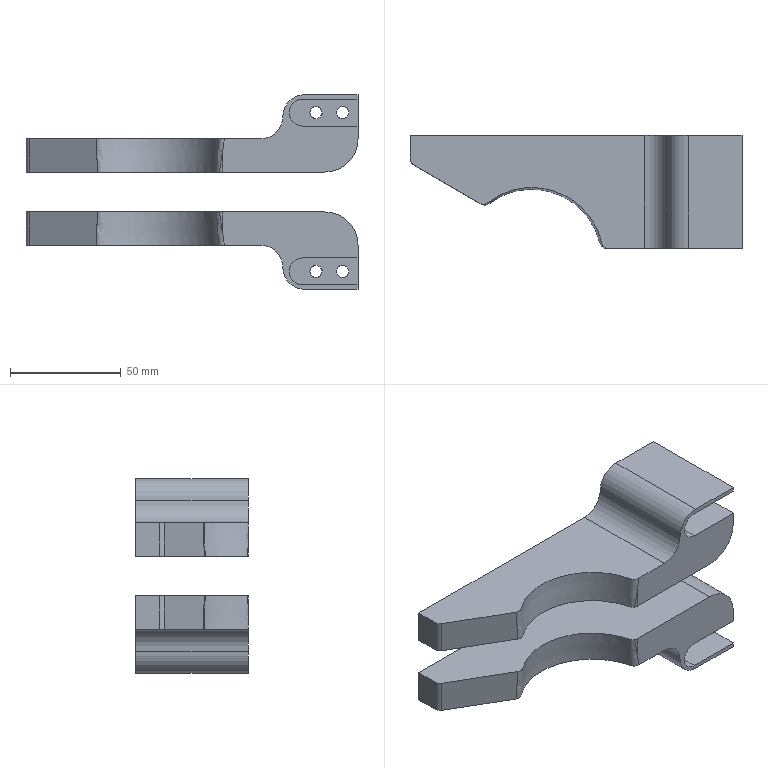NC program | NX | posted with a generic post | part box 150 x 51 x 88 mm
Lines 43 to 1068 of 21230:
(ADAPTIVE_MILLING_COPY , TOOL : D12C)
N72 T12 M6
N74 G54
N76 G17 G0 G90 X-87.243 Y2.564 S9500 M3
N78 G43 Z30. H12
N80 Z-14.
N82 G94 G1 Z-17. F1000.
N84 X-85.489 Y2.014 F3000.
N86 G3 X-84.076 Y2.564 R1.22
N88 X-83.366 Y5.337 R7.621
N90 X-83.032 Y14.477 R92.487
N92 G2 X-82.959 Y17.999 R38.072
N94 X-79.583 Y22.839 R7.317
N96 X-73.241 Y24.982 R15.248
N98 X-63.509 Y25.457 R81.144
N100 G1 X-62.234 Y25.466
N102 X-60.584 Y25.474
N104 X-58.409 Y25.479
N106 X-55.034 Y25.483
N108 X-47.909 Y25.485
N110 X74.716 Y25.478
N112 X74.791 Y25.477
N114 X74.941 Y25.472
N116 X75.091 Y25.462
N118 G2 X80.055 Y22.427 R7.028
N120 X82.397 Y16.243 R14.195
N122 X82.947 Y7.042 R66.047
N124 G1 X82.959 Y5.918
N126 X82.968 Y4.568
N128 X82.976 Y2.843
N130 X82.982 Y0.593
N132 X82.986 Y-2.932
N134 X82.988 Y-10.957
N136 G2 X82.946 Y-17.856 R138.275
N138 X79.66 Y-22.754 R7.252
N140 X73.342 Y-24.96 R14.994
N142 X64.586 Y-25.446 R70.223
N144 G1 X63.461 Y-25.458
N146 X62.111 Y-25.467
N148 X60.536 Y-25.475
N150 X58.286 Y-25.48
N152 X54.911 Y-25.484
N154 X47.561 Y-25.486
N156 X-74.689 Y-25.485
N158 X-74.764
N160 X-74.839 Y-25.483
N162 X-74.988 Y-25.476
N164 X-75.138 Y-25.465
N166 G2 X-80.128 Y-22.335 R7.093
N168 X-82.394 Y-16.278 R14.265
N170 X-82.95 Y-7.078 R64.861
N172 X-82.909 Y0.045 R99.947
N174 G3 X-82.049 Y14.411 R129.844
N176 G2 X-81.128 Y17.792 R9.852
N178 X-76.298 Y23.504 R6.212
N180 X-62.095 Y24.43 R100.62
N182 G1 X-60.82 Y24.443
N184 X-59.32 Y24.453
N186 X-57.52 Y24.461
N188 X-55.12 Y24.467
N190 X-51.595 Y24.471
N192 X-44.92 Y24.473
N194 X71.33 Y24.467
N196 X71.48 Y24.466
N198 X71.705 Y24.458
N200 X71.855 Y24.451
N202 G2 X78.937 Y20.113 R9.119
N204 X81.352 Y13.152 R17.438
N206 X81.922 Y3.726 R73.479
N208 X81.951 Y-14.498 R846.878
N210 X81.136 Y-17.623 R10.548
N212 X76.298 Y-23.504 R6.215
N214 X61.795 Y-24.434 R102.394
N216 G1 X60.595 Y-24.445
N218 X59.02 Y-24.455
N220 X57.145 Y-24.463
N222 X54.595 Y-24.469
N224 X50.77 Y-24.473
N226 X42.745 Y-24.475
N228 X-71.33 Y-24.474
N230 X-71.48 Y-24.472
N232 X-71.705 Y-24.465
N234 X-71.855 Y-24.458
N236 G2 X-78.938 Y-20.121 R9.12
N238 X-81.361 Y-13.085 R17.42
N240 X-81.615 Y2.256 R70.947
N242 G3 X-81.146 Y17.535 R168.471
N244 G1 X-81.129 Y17.684
N246 X-81.146 Y17.535
N248 X-81.15 Y17.465
N250 Y11.278
N252 G2 X-81.277 Y-2.863 R390.887
N254 G3 X-80.682 Y-12.884 R63.102
N256 X-78.284 Y-19.291 R15.229
N258 X-72.558 Y-23.014 R9.886
N260 X-65.493 Y-23.797 R31.227
N262 X-51.093 Y-23.867 R747.498
N264 G1 X-11.568 Y-23.868
N266 X-11.193 Y-23.869
N268 X54.282 Y-23.87
N270 X59.682 Y-23.846
N272 G3 X68.172 Y-23.65 R287.309
N274 G1 X74.965
N276 X75.035 Y-23.646
N278 X74.965 Y-23.65
N280 X51.025
N282 X50.975 Y-23.648
N284 G2 X46.571 Y-23.171 R50.175
N286 G3 X36.303 Y-22.893 R128.49
N288 G1 X34.053 Y-22.887
N290 X30.528 Y-22.883
N292 X22.578 Y-22.881
N294 X-7.947
N296 X-8.697 Y-22.877
N298 X-9.747 Y-22.875
N300 X-10.197
N302 X-11.022 Y-22.872
N304 X-11.847
N306 X-12.897 Y-22.87
N308 X-13.722 Y-22.871
N310 X-14.622 Y-22.869
N312 X-15.822 Y-22.87
N314 X-16.497 Y-22.869
N316 X-17.772 Y-22.87
N318 X-18.222
N320 X-18.972 Y-22.869
N322 X-20.022 Y-22.87
N324 X-20.772 Y-22.868
N326 X-22.047 Y-22.87
N328 X-23.022 Y-22.867
N330 X-24.147 Y-22.87
N332 X-24.897 Y-22.868
N334 X-25.872 Y-22.869
N336 X-26.397
N338 X-27.147 Y-22.867
N340 X-27.897 Y-22.868
N342 X-29.247 Y-22.866
N344 X-29.697
N346 X-30.597 Y-22.868
N348 X-31.572 Y-22.866
N350 X-32.472 Y-22.868
N352 X-33.222 Y-22.867
N354 X-34.497 Y-22.869
N356 X-35.547 Y-22.866
N358 X-36.522 Y-22.868
N360 X-37.497 Y-22.867
N362 X-38.472 Y-22.869
N364 X-39.522 Y-22.866
N366 X-40.497 Y-22.868
N368 X-41.547 Y-22.866
N370 X-42.447 Y-22.868
N372 X-43.272 Y-22.867
N374 X-44.397 Y-22.869
N376 X-45.222 Y-22.867
N378 X-46.197 Y-22.868
N380 X-47.172 Y-22.866
N382 X-47.922 Y-22.867
N384 X-49.197 Y-22.866
N386 X-49.647 Y-22.865
N388 X-50.322 Y-22.867
N390 X-51.297 Y-22.865
N392 X-51.822 Y-22.866
N394 X-52.497 Y-22.867
N396 X-53.547 Y-22.865
N398 X-54.222 Y-22.866
N400 X-55.347 Y-22.864
N402 X-55.797 Y-22.863
N404 G2 X-67.343 Y-22.645 R181.656
N406 X-72.93 Y-21.333 R15.227
N408 X-78.322 Y-15.229 R11.546
N410 X-79.985 Y-7.412 R25.774
N412 X-80.19 Y-0.893 R100.233
N414 G1 X-80.206 Y-0.82
N416 X-80.226 Y-0.748
N418 X-80.251 Y-0.677
N420 X-80.279 Y-0.607
N422 X-80.31 Y-0.539
N424 X-80.324 Y-0.514
N426 X-80.364 Y-0.45
N428 G2 X-79.856 Y-2.236 R3.949
N430 G3 X-79.127 Y-9.247 R243.86
N432 X-76.81 Y-16.247 R18.289
N434 X-69.838 Y-21.221 R11.574
N436 X-62.639 Y-22.142 R31.464
N438 X-40.815 Y-22.267 R842.14
N440 G1 X-39.99 Y-22.265
N442 X-38.715 Y-22.268
N444 X-38.265 Y-22.267
N446 X-36.615 Y-22.27
N448 X-35.715 Y-22.267
N450 X-35.19 Y-22.268
N452 X-33.69 Y-22.265
N454 X-32.865 Y-22.267
N456 X-32.19 Y-22.266
N458 X-31.665 Y-22.267
N460 X-31.14 Y-22.266
N462 X-30.765 Y-22.267
N464 X-29.565 Y-22.265
N466 X-29.04 Y-22.266
N468 X-26.94 Y-22.265
N470 X-26.415 Y-22.266
N472 X-25.59 Y-22.265
N474 X-24.99 Y-22.267
N476 X-23.115 Y-22.265
N478 X-22.29 Y-22.267
N480 X-21.84
N482 X-20.49 Y-22.27
N484 X-19.215 Y-22.268
N486 X-18.165 Y-22.27
N488 X-16.965 Y-22.268
N490 X-15.99 Y-22.27
N492 X-15.24 Y-22.269
N494 X-14.79
N496 X-13.365 Y-22.268
N498 X-12.84 Y-22.27
N500 X-11.19
N502 X-10.365 Y-22.274
N504 X6.66 Y-22.275
N506 X7.035 Y-22.276
N508 X27.36 Y-22.277
N510 X27.735 Y-22.278
N512 X29.61
N514 X30.06 Y-22.28
N516 G2 X44.607 Y-22.472 R319.497
N518 X46.058 Y-22.871 R3.551
N520 G1 X48.391 Y-23.431
N522 X46.058 Y-22.871
N524 X45.964 Y-22.841
N526 X45.278 Y-22.557
N528 G3 X41.134 Y-21.605 R12.134
N530 X30.791 Y-21.305 R135.44
N532 G1 X28.766 Y-21.297
N534 X26.666 Y-21.292
N536 X22.541 Y-21.289
N538 X10.241 Y-21.287
N540 X9.491 Y-21.284
N542 X8.441 Y-21.282
N544 X7.541 Y-21.283
N546 X6.941 Y-21.281
N548 X5.591 Y-21.28
N550 X4.841
N552 X4.016 Y-21.277
N554 X3.116 Y-21.278
N556 X2.216 Y-21.276
N558 X1.241 Y-21.277
N560 X0.266 Y-21.275
N562 X-0.559 Y-21.276
N564 X-1.684 Y-21.274
N566 X-2.584 Y-21.276
N568 X-3.334 Y-21.275
N570 X-4.609 Y-21.276
N572 X-5.059 Y-21.277
N574 X-5.959 Y-21.274
N576 X-6.784 Y-21.276
N578 X-7.534 Y-21.274
N580 X-8.059 Y-21.272
N582 X-9.034 Y-21.273
N584 X-9.709 Y-21.272
N586 X-10.984
N588 X-11.959 Y-21.27
N590 X-12.859 Y-21.271
N592 X-13.909 Y-21.27
N594 X-15.034 Y-21.272
N596 X-16.084 Y-21.269
N598 X-17.209 Y-21.271
N600 X-18.559 Y-21.268
N602 X-19.234
N604 X-21.034 Y-21.266
N606 X-22.384 Y-21.263
N608 X-23.134 Y-21.265
N610 X-24.259 Y-21.264
N612 X-24.709 Y-21.263
N614 X-25.609 Y-21.266
N616 X-26.659 Y-21.264
N618 X-27.634 Y-21.267
N620 X-28.459 Y-21.265
N622 X-29.659 Y-21.267
N624 X-30.634 Y-21.265
N626 X-31.984 Y-21.269
N628 X-32.659 Y-21.268
N630 X-33.934 Y-21.269
N632 X-34.459 Y-21.27
N634 X-35.209 Y-21.268
N636 X-36.409 Y-21.269
N638 X-37.159 Y-21.267
N640 X-38.284 Y-21.268
N642 X-39.034 Y-21.266
N644 G2 X-61.083 Y-21.154 R945.044
N646 X-68.437 Y-20.266 R31.428
N648 X-76.39 Y-13.29 R12.118
N650 X-78.285 Y-6.06 R26.581
N652 G3 X-78.953 Y-2.299 R26.649
N654 X-79.846 Y-1.274 R5.85
N656 G1 X-79.926 Y-1.147
N658 X-79.846 Y-1.274
N660 X-79.758 Y-1.385
N662 X-79.157 Y-1.986
N664 G2 X-78.348 Y-3.652 R3.593
N666 X-77.085 Y-9.056 R710.487
N668 G3 X-73.818 Y-15.647 R15.927
N670 X-66.765 Y-19.673 R13.495
N672 X-58.503 Y-20.557 R39.762
N674 X-36.154 Y-20.668 R982.402
N676 G1 X-35.629 Y-20.669
N678 X-35.029 Y-20.667
N680 X-34.279 Y-20.669
N682 X-33.604 Y-20.667
N684 X-31.954 Y-20.67
N686 X-30.904 Y-20.667
N688 X-30.379 Y-20.668
N690 X-28.729 Y-20.664
N692 X-28.279
N694 X-27.304 Y-20.663
N696 X-25.804 Y-20.666
N698 X-24.679 Y-20.663
N700 X-23.929 Y-20.665
N702 X-23.554
N704 X-22.504 Y-20.667
N706 X-21.754 Y-20.666
N708 X-21.379 Y-20.667
N710 X-20.704
N712 X-20.029 Y-20.669
N714 X-18.004 Y-20.667
N716 X-17.404 Y-20.669
N718 X-16.579 Y-20.668
N720 X-15.454 Y-20.671
N722 X-14.854 Y-20.669
N724 X-13.129 Y-20.673
N726 X-12.379 Y-20.671
N728 X-11.104 Y-20.674
N730 X-10.354 Y-20.673
N732 X-9.604 Y-20.675
N734 X-8.329 Y-20.673
N736 X-7.279 Y-20.675
N738 X-6.754
N740 X-5.929 Y-20.677
N742 X-5.404 Y-20.676
N744 X-4.804 Y-20.677
N746 X-3.904 Y-20.675
N748 X-3.379 Y-20.676
N750 X-2.104 Y-20.674
N752 X-1.354 Y-20.676
N754 X-0.529 Y-20.675
N756 X0.896 Y-20.678
N758 X1.721 Y-20.677
N760 X2.396 Y-20.679
N762 X3.821 Y-20.677
N764 X5.246 Y-20.681
N766 X6.371 Y-20.68
N768 X8.546 Y-20.686
N770 X9.596 Y-20.685
N772 X10.121 Y-20.686
N774 X11.321 Y-20.685
N776 X11.846 Y-20.686
N778 X12.971 Y-20.685
N780 X13.496 Y-20.687
N782 X14.621 Y-20.685
N784 X15.146 Y-20.687
N786 X16.271 Y-20.685
N788 X16.796 Y-20.687
N790 X17.771 Y-20.686
N792 X18.296 Y-20.687
N794 X19.271 Y-20.686
N796 X19.871 Y-20.688
N798 X20.771 Y-20.686
N800 X21.371 Y-20.688
N802 X22.121 Y-20.687
N804 X22.796 Y-20.689
N806 X23.471 Y-20.688
N808 X24.296 Y-20.691
N810 X24.821 Y-20.69
N812 G2 X39.293 Y-20.912 R296.11
N814 X42.782 Y-21.357 R16.806
N816 G1 X42.85 Y-21.389
N818 G2 X43.39 Y-22.691 R1.208
N820 X42.659 Y-23.536 Z-16.952 R1.255
N822 G1 X41.549 Y-24.09 Z-16.9
N824 X39.568 Y-25.08
N826 X39.306 Y-25.171
N828 X39.032 Y-25.207
N830 X-48.718
N832 G2 X-62.14 Y-24.181 R88.992
N834 G1 X-64.415 Y-23.833
N836 X-66.686 Y-23.465
N838 G2 X-72.757 Y-21.437 R25.318
N840 X-75.806 Y-19.088 R10.097
N842 X-80.215 Y-11.344 R22.758
N844 G1 X-81.751 Y-6.768
N846 G2 X-81.788 Y-6.143 R1.263
N848 G1 X-81.354 Y-4.047
N850 X-81.045 Y-2.599 Z-16.962
N852 G2 X-80.491 Y-1.896 Z-17. R1.202
N854 X-79.051 Y-2.092 R1.208
N856 X-77.872 Y-4.165 R4.889
N858 G3 X-76.228 Y-9.621 R527.122
N860 X-66.858 Y-18.672 R13.678
N862 X-58.719 Y-19.873 R33.096
N864 X-40.121 Y-20.063 R474.803
N866 G1 X-38.996 Y-20.066
N868 X-38.546
N870 X-38.021 Y-20.067
N872 X-37.646 Y-20.066
N874 X-36.521 Y-20.069
N876 X-35.996 Y-20.068
N878 X-35.246 Y-20.07
N880 X-34.796 Y-20.069
N882 X-34.196
N884 X-33.521 Y-20.068
N886 X-32.921
N888 X-32.471
N890 X-32.171
N892 X-31.196 Y-20.065
N894 X-30.596 Y-20.066
N896 X-29.621 Y-20.064
N898 X-28.571 Y-20.066
N900 X-27.071 Y-20.063
N902 X-26.546
N904 X-26.021
N906 X-25.571 Y-20.064
N908 X-25.121
N910 X-24.671
N912 X-24.221
N914 X-23.771 Y-20.065
N916 X-23.246 Y-20.064
N918 X-22.271 Y-20.067
N920 X-20.471 Y-20.064
N922 X-19.871 Y-20.066
N924 X-19.046 Y-20.065
N926 X-18.446
N928 X-17.846 Y-20.067
N930 X-17.246
N932 X-16.871 Y-20.068
N934 X-16.346
N936 X-15.521 Y-20.07
N938 X-14.921 Y-20.069
N940 X-13.496 Y-20.073
N942 X-12.971 Y-20.072
N944 X-12.221 Y-20.074
N946 X-10.646 Y-20.071
N948 X-9.146 Y-20.075
N950 X-8.696
N952 X-8.246 Y-20.076
N954 X-7.646 Y-20.075
N956 X-7.196 Y-20.076
N958 X-6.596 Y-20.075
N960 X-5.621 Y-20.077
N962 X-4.421 Y-20.074
N964 X-3.896 Y-20.076
N966 X-2.696 Y-20.074
N968 X-1.346 Y-20.077
N970 X-0.821
N972 X-0.071 Y-20.079
N974 X1.429 Y-20.076
N976 X2.779 Y-20.08
N978 X3.379 Y-20.081
N980 X4.054 Y-20.08
N982 X6.079 Y-20.085
N984 X7.279 Y-20.083
N986 X7.879 Y-20.085
N988 X9.004 Y-20.083
N990 X9.604 Y-20.085
N992 X10.654 Y-20.083
N994 X11.404 Y-20.085
N996 X12.079 Y-20.086
N998 X12.529
N1000 X12.904 Y-20.087
N1002 X13.879 Y-20.085
N1004 X14.404
N1006 X15.304 Y-20.084
N1008 X15.829 Y-20.085
N1010 X16.504 Y-20.084
N1012 X17.554 Y-20.087
N1014 X18.379 Y-20.085
N1016 X19.129 Y-20.087
N1018 X19.879 Y-20.086
N1020 X20.329 Y-20.087
N1022 X20.929 Y-20.086
N1024 X22.054 Y-20.09
N1026 X22.504 Y-20.089
N1028 X23.104 Y-20.091
N1030 X23.629
N1032 X25.429 Y-20.097
N1034 G2 X39.149 Y-20.345 R236.141
N1036 X41.671 Y-20.679 R12.656
N1038 G1 X41.74 Y-20.71
N1040 X41.759 Y-20.72
N1042 X41.887 Y-20.798
N1044 G3 X38.785 Y-19.698 R7.337
N1046 X30.709 Y-19.168 R56.952
N1048 X10.535 Y-19.087 R993.782
N1050 G1 X9.935 Y-19.085
N1052 X8.96 Y-19.086
N1054 X7.91 Y-19.084
N1056 X7.235
N1058 X6.035 Y-19.081
N1060 X5.285 Y-19.082
N1062 X4.16 Y-19.079
N1064 X3.035 Y-19.081
N1066 X2.21 Y-19.079
N1068 X1.085
N1070 X0.26 Y-19.077
N1072 X-0.415
N1074 X-0.94 Y-19.078
N1076 X-1.615 Y-19.077
N1078 X-2.74 Y-19.078
N1080 X-3.265 Y-19.077
N1082 X-3.865 Y-19.076
N1084 X-5.065 Y-19.078
N1086 X-5.89 Y-19.076
N1088 X-6.865 Y-19.077
N1090 X-7.615 Y-19.075
N1092 X-8.815
N1094 X-9.415 Y-19.076
N1096 X-10.09 Y-19.074
N1098 X-11.29 Y-19.075
N1100 X-12.115 Y-19.072
N1102 X-13.015
N1104 X-13.915 Y-19.07
N1106 X-14.74 Y-19.071
N1108 X-15.715 Y-19.069
N1110 X-16.915 Y-19.07
N1112 X-17.665 Y-19.068
N1114 X-18.49
N1116 X-18.94
N1118 X-19.765 Y-19.067
N1120 X-20.815 Y-19.068
N1122 X-22.015 Y-19.064
N1124 X-22.69 Y-19.065
N1126 X-24.415 Y-19.063
N1128 X-24.865 Y-19.062
N1130 X-25.69 Y-19.064
N1132 X-26.665
N1134 X-27.79 Y-19.066
N1136 X-28.54 Y-19.065
N1138 X-29.74 Y-19.067
N1140 X-30.565 Y-19.066
N1142 X-31.54 Y-19.068
N1144 X-32.815 Y-19.066
N1146 X-33.49 Y-19.067
N1148 X-34.84 Y-19.066
N1150 X-35.59 Y-19.065
N1152 X-36.19 Y-19.066
N1154 G2 X-56.964 Y-18.905 R702.792
N1156 X-65.201 Y-17.843 R35.687
N1158 X-74.303 Y-10.272 R13.986
N1160 X-76.516 Y-4.941 R71.765
N1162 G3 X-77.48 Y-3.174 R5.72
N1164 G1 X-77.538 Y-3.125
N1166 X-77.598 Y-3.08
N1168 X-77.665 Y-3.034
N1170 X-77.728 Y-3.003
N1172 X-78.774 Y-2.346
N1174 X-78.885 Y-2.258
N1176 X-78.774 Y-2.346
N1178 X-77.728 Y-3.003
N1180 X-77.665 Y-3.034
N1182 G2 X-76.561 Y-4.22 R2.771
N1184 X-74.378 Y-8.66 R66.723
N1186 G3 X-68.8 Y-15.187 R15.611
N1188 X-61.05 Y-17.829 R19.574
N1190 X-50.123 Y-18.413 R86.047
N1192 G1 X-48.773 Y-18.426
N1194 X-47.348 Y-18.436
N1196 X-46.373 Y-18.441
N1198 X-45.998 Y-18.444
N1200 X-43.223 Y-18.453
N1202 X-40.298 Y-18.459
N1204 X-37.373 Y-18.461
N1206 X-37.148
N1208 X-36.698 Y-18.463
N1210 X-23.648 Y-18.461
N1212 X-23.048 Y-18.463
N1214 X-22.223 Y-18.462
N1216 X-21.248 Y-18.466
N1218 X-20.723 Y-18.465
N1220 X-20.198 Y-18.467
N1222 X-19.898 Y-18.466
N1224 X-19.148 Y-18.468
N1226 X-18.023 Y-18.467
N1228 X-16.973 Y-18.47
N1230 X-16.223 Y-18.468
N1232 X-15.173 Y-18.471
N1234 X-14.498 Y-18.47
N1236 X-13.448 Y-18.473
N1238 X-12.473 Y-18.472
N1240 X-11.648 Y-18.474
N1242 X-10.298 Y-18.472
N1244 X-9.173 Y-18.476
N1246 X-8.123 Y-18.474
N1248 X-7.373 Y-18.476
N1250 X-6.098 Y-18.474
N1252 X-5.348 Y-18.476
N1254 X-3.998 Y-18.474
N1256 X-3.173 Y-18.477
N1258 X-2.648
N1260 X-2.423
N1262 X-2.048
N1264 X-1.298 Y-18.478
N1266 X-0.698 Y-18.477
N1268 X0.652 Y-18.481
N1270 X1.177 Y-18.48
N1272 X6.502 Y-18.487
N1274 X11.827 Y-18.49
N1276 X16.252
N1278 X16.777 Y-18.492
N1280 G2 X33.8 Y-18.677 R525.349
N1282 X39.956 Y-19.492 R26.893
N1284 G1 X40.536 Y-19.736
N1286 X41.47 Y-20.533
N1288 X41.53 Y-20.577
N1290 X41.47 Y-20.533
N1292 X40.536 Y-19.736
N1294 G3 X37.856 Y-18.464 R5.88
N1296 X30.788 Y-17.673 R35.69
N1298 X6.414 Y-17.488 R889.918
N1300 G1 X5.139
N1302 X4.614
N1304 X4.014 Y-17.486
N1306 X2.889 Y-17.485
N1308 X2.514
N1310 X1.914 Y-17.483
N1312 X0.939
N1314 X0.564
N1316 X-0.186 Y-17.48
N1318 X-1.086
N1320 X-1.461
N1322 X-2.061 Y-17.479
N1324 X-3.186
N1326 X-3.936 Y-17.481
N1328 X-4.986 Y-17.477
N1330 X-5.811
N1332 X-7.011 Y-17.475
N1334 X-7.461 Y-17.474
N1336 X-8.286 Y-17.475
N1338 X-9.486 Y-17.473
N1340 X-10.386 Y-17.474
N1342 X-11.361 Y-17.472
N1344 X-12.261 Y-17.473
N1346 X-13.386 Y-17.47
N1348 X-14.211 Y-17.471
N1350 X-15.186 Y-17.469
N1352 X-16.086 Y-17.47
N1354 X-16.986 Y-17.468
N1356 X-17.436 Y-17.467
N1358 X-18.261 Y-17.468
N1360 X-19.311 Y-17.465
N1362 X-20.211 Y-17.466
N1364 X-21.111 Y-17.463
N1366 X-22.236 Y-17.465
N1368 X-22.911 Y-17.463
N1370 X-24.111 Y-17.464
N1372 X-24.711 Y-17.465
N1374 X-25.311 Y-17.463
N1376 X-26.511 Y-17.464
N1378 X-27.111 Y-17.465
N1380 X-27.786 Y-17.463
N1382 X-28.686 Y-17.464
N1384 X-29.136
N1386 X-30.111 Y-17.462
N1388 X-31.086 Y-17.464
N1390 X-32.061 Y-17.462
N1392 X-32.886 Y-17.463
N1394 X-34.086 Y-17.461
N1396 X-34.836 Y-17.462
N1398 X-36.036 Y-17.46
N1400 X-36.711 Y-17.461
N1402 X-37.761 Y-17.459
N1404 X-38.286 Y-17.458
N1406 X-39.036 Y-17.459
N1408 X-40.236 Y-17.455
N1410 G2 X-56.282 Y-17.205 R327.82
N1412 X-64.452 Y-15.765 R29.286
N1414 X-72.422 Y-9.235 R15.718
N1416 G3 X-75.235 Y-4.627 R451.065
N1418 X-76.316 Y-3.511 R2.906
N1420 G1 X-76.386 Y-3.484
N1422 X-76.435 Y-3.472
N1424 X-77.601 Y-3.064
N1426 X-76.435 Y-3.472
N1428 X-76.386 Y-3.484
N1430 G2 X-75.064 Y-4.446 R2.599
N1432 X-72.448 Y-8.104 R43.318
N1434 G3 X-65.427 Y-14.364 R17.563
N1436 X-57.246 Y-16.411 R24.786
N1438 X-44.733 Y-16.831 R145.448
N1440 G1 X-43.158 Y-16.839
N1442 X-40.908 Y-16.847
N1444 X-37.833 Y-16.853
N1446 X-36.258 Y-16.854
N1448 X-35.733 Y-16.857
N1450 X-34.533
N1452 X-33.558 Y-16.86
N1454 X-32.583 Y-16.859
N1456 X-31.308 Y-16.863
N1458 X-30.783 Y-16.862
N1460 X-29.358 Y-16.865
N1462 X-28.908 Y-16.864
N1464 X-28.083 Y-16.866
N1466 X-27.483 Y-16.865
N1468 X-26.958 Y-16.866
N1470 X-26.283 Y-16.864
N1472 X-25.383 Y-16.865
N1474 X-25.008 Y-16.864
N1476 X-24.408 Y-16.865
N1478 X-23.883 Y-16.864
N1480 X-22.083 Y-16.867
N1482 X-21.483 Y-16.866
N1484 X-20.883 Y-16.868
N1486 X-19.608 Y-16.866
N1488 X-19.008 Y-16.867
N1490 X-17.583 Y-16.866
N1492 X-16.458 Y-16.869
N1494 X-15.933 Y-16.868
N1496 X-15.258 Y-16.87
N1498 X-14.733
N1500 X-14.358 Y-16.871
N1502 X-13.758
N1504 X-13.158 Y-16.872
N1506 X-11.658 Y-16.871
N1508 X-10.608 Y-16.874
N1510 X-9.783 Y-16.872
N1512 X-9.033 Y-16.875
N1514 X-8.358 Y-16.874
N1516 X-7.983 Y-16.875
N1518 X-7.458
N1520 X-6.258 Y-16.879
N1522 X-5.283 Y-16.877
N1524 X-4.533 Y-16.879
N1526 X-4.158 Y-16.878
N1528 X-3.633 Y-16.879
N1530 X-2.958 Y-16.878
N1532 X-1.533 Y-16.882
N1534 X-0.708 Y-16.88
N1536 X0.192 Y-16.883
N1538 X0.642 Y-16.882
N1540 X1.542 Y-16.885
N1542 X1.767 Y-16.884
N1544 X2.592 Y-16.887
N1546 X3.417 Y-16.886
N1548 X4.842 Y-16.89
N1550 X5.892 Y-16.888
N1552 X6.717 Y-16.891
N1554 X7.917 Y-16.89
N1556 X8.742 Y-16.893
N1558 X9.192
N1560 X9.717 Y-16.895
N1562 G2 X30.266 Y-17.076 R737.854
N1564 X37.555 Y-17.905 R36.001
N1566 X39.316 Y-18.61 R4.647
N1568 G1 X39.548 Y-18.882
N1570 X39.618 Y-18.952
N1572 X39.548 Y-18.882
N1574 X39.316 Y-18.61
N1576 G3 X37.099 Y-17.272 R4.626
N1578 X30.528 Y-16.209 R26.301
N1580 X16.208 Y-15.923 R271.7
N1582 G1 X12.533 Y-15.911
N1584 X8.858 Y-15.904
N1586 X7.058 Y-15.901
N1588 X6.458 Y-15.898
N1590 X5.108 Y-15.894
N1592 X3.908 Y-15.893
N1594 X3.233 Y-15.89
N1596 X2.483 Y-15.889
N1598 X1.658
N1600 X0.683 Y-15.885
N1602 X-0.517
N1604 X-1.192 Y-15.883
N1606 X-2.467
N1608 X-3.217 Y-15.884
N1610 X-4.342 Y-15.879
N1612 X-5.767 Y-15.881
N1614 X-6.442 Y-15.879
N1616 X-8.317 Y-15.877
N1618 X-10.117
N1620 X-10.942 Y-15.875
N1622 X-12.217
N1624 X-12.967 Y-15.873
N1626 X-14.092
N1628 X-14.917 Y-15.87
N1630 X-16.117 Y-15.871
N1632 X-16.867 Y-15.869
N1634 X-18.067
N1636 X-18.817 Y-15.868
N1638 X-20.017 Y-15.869
N1640 X-20.767 Y-15.867
N1642 X-21.892
N1644 X-22.417 Y-15.868
N1646 X-23.242 Y-15.866
N1648 X-24.442 Y-15.867
N1650 X-25.267 Y-15.865
N1652 X-26.392 Y-15.867
N1654 X-27.292 Y-15.864
N1656 X-28.267 Y-15.865
N1658 X-29.467 Y-15.862
N1660 X-30.517 Y-15.863
N1662 X-31.417 Y-15.861
N1664 X-32.317
N1666 X-32.692
N1668 X-33.517 Y-15.858
N1670 G2 X-52.715 Y-15.661 R562.015
N1672 X-61.391 Y-14.49 R38.128
N1674 X-70.647 Y-8.288 R18.296
N1676 G3 X-73.895 Y-4.456 R64.699
N1678 X-75.072 Y-3.642 R2.732
N1680 G1 X-76.298 Y-3.504
N1682 X-75.072 Y-3.642
N1684 G2 X-73.541 Y-4.448 R2.919
N1686 X-70.206 Y-7.895 R44.507
N1688 G3 X-58.391 Y-14.349 R20.169
N1690 X-48.834 Y-15.138 R61.06
N1692 X-25.809 Y-15.263 R963.1
N1694 G1 X-24.609 Y-15.266
N1696 X-23.934 Y-15.267
N1698 X-23.334 Y-15.266
N1700 X-22.659 Y-15.267
N1702 X-21.159 Y-15.265
N1704 X-20.334 Y-15.268
N1706 X-19.284 Y-15.266
N1708 X-18.759 Y-15.267
N1710 X-16.959 Y-15.266
N1712 X-16.359 Y-15.269
N1714 X-15.234 Y-15.268
N1716 X-14.484 Y-15.271
N1718 X-13.809
N1720 X-12.384 Y-15.275
N1722 X-11.859 Y-15.276
N1724 X-9.234 Y-15.28
N1726 X-6.609 Y-15.281
N1728 X-5.109 Y-15.279
N1730 X-4.734 Y-15.28
N1732 X-3.984
N1734 X-2.634 Y-15.284
N1736 X-0.609 Y-15.288
N1738 X0.366 Y-15.287
N1740 X2.466 Y-15.293
N1742 X2.916 Y-15.292
N1744 X5.166 Y-15.3
N1746 X5.841 Y-15.299
N1748 X6.666 Y-15.302
N1750 X7.266 Y-15.301
N1752 X8.316 Y-15.305
N1754 G2 X28.113 Y-15.511 R641.52
N1756 X35.919 Y-16.437 R38.174
N1758 X38.267 Y-17.397 R7.39
N1760 G1 X38.325 Y-17.45
N1762 X39.153 Y-18.42
N1764 X38.325 Y-17.45
N1766 G3 X35.901 Y-15.885 R5.175
N1768 X29.128 Y-14.685 R26.056
N1770 X15.934 Y-14.346 R213.437
N1772 G1 X12.934 Y-14.331
N1774 X9.859 Y-14.32
N1776 X7.61 Y-14.315
N1778 X6.86 Y-14.309
N1780 X5.885 Y-14.306
N1782 X5.285 Y-14.305
N1784 X4.535 Y-14.302
N1786 X3.335 Y-14.299
N1788 X2.51 Y-14.298
N1790 X1.61 Y-14.293
N1792 X0.86
N1794 X-0.115 Y-14.289
N1796 X-0.565 Y-14.287
N1798 X-1.615
N1800 X-2.365 Y-14.285
N1802 X-3.34
N1804 X-3.865 Y-14.284
N1806 X-4.465 Y-14.283
N1808 X-5.59 Y-14.284
N1810 X-6.49 Y-14.281
N1812 X-7.465 Y-14.282
N1814 X-8.515 Y-14.279
N1816 X-9.265
N1818 X-10.39 Y-14.277
N1820 X-11.44
N1822 X-12.265 Y-14.274
N1824 X-13.09
N1826 X-13.465
N1828 X-14.215 Y-14.271
N1830 X-15.49
N1832 X-16.39 Y-14.269
N1834 X-17.215 Y-14.27
N1836 X-18.265 Y-14.268
N1838 X-19.465 Y-14.27
N1840 X-20.215 Y-14.268
N1842 X-21.34 Y-14.269
N1844 X-21.865 Y-14.268
N1846 X-22.69 Y-14.266
N1848 X-23.665 Y-14.267
N1850 X-24.415 Y-14.265
N1852 X-25.165
N1854 X-25.765 Y-14.266
N1856 X-26.665 Y-14.264
N1858 X-27.64 Y-14.266
N1860 X-28.54 Y-14.264
N1862 X-29.44
N1864 X-30.265 Y-14.262
N1866 X-30.79 Y-14.261
N1868 G2 X-50.738 Y-14.042 R580.247
N1870 X-59.711 Y-12.826 R40.132
N1872 X-68.81 Y-7.506 R21.61
N1874 G3 X-72.625 Y-4.127 R41.66
N1876 X-73.677 Y-3.65 R2.203
N1878 G1 X-74.965
N1880 X-73.677
N1882 G2 X-71.883 Y-4.336 R3.259
N1884 X-68.075 Y-7.375 R49.304
N1886 G3 X-55.189 Y-12.954 R24.096
N1888 X-44.038 Y-13.579 R91.815
N1890 X-24.839 Y-13.666 R951.618
N1892 G1 X-22.814 Y-13.665
N1894 X-21.914 Y-13.668
N1896 X-21.239 Y-13.666
N1898 X-20.789 Y-13.668
N1900 X-20.414 Y-13.667
N1902 X-19.514 Y-13.669
N1904 X-18.689 Y-13.668
N1906 X-18.164 Y-13.669
N1908 X-16.964 Y-13.668
N1910 X-15.764 Y-13.671
N1912 X-14.864 Y-13.67
N1914 X-13.889 Y-13.674
N1916 X-13.214 Y-13.673
N1918 X-11.939 Y-13.677
N1920 X-10.739 Y-13.676
N1922 X-10.289 Y-13.678
N1924 X-8.564 Y-13.677
N1926 X-7.964 Y-13.679
N1928 X-7.289
N1930 X-6.239 Y-13.682
N1932 X-4.889 Y-13.681
N1934 X-4.064 Y-13.684
N1936 X-3.389 Y-13.683
N1938 X-0.989 Y-13.691
N1940 X-0.539 Y-13.692
N1942 X0.136 Y-13.694
N1944 X0.586 Y-13.695
N1946 X4.711 Y-13.707
N1948 X8.836 Y-13.715
N1950 X9.511 Y-13.719
N1952 G2 X27.357 Y-14.002 R404.679
N1954 X34.842 Y-15.057 R34.534
N1956 X37.473 Y-16.288 R7.135
N1958 G1 X37.523 Y-16.344
N1960 X37.558 Y-16.378
N1962 X37.908 Y-16.95
N1964 X37.967 Y-17.03
N1966 X37.908 Y-16.95
N1968 X37.558 Y-16.378
N1970 G3 X35.674 Y-14.833 R4.053
N1972 X29.958 Y-13.369 R18.955
N1974 X18.653 Y-12.803 R107.829
N1976 G1 X17.228 Y-12.786
N1978 X15.578 Y-12.77
N1980 X13.253 Y-12.752
N1982 X10.928 Y-12.738
N1984 X8.603 Y-12.728
N1986 X6.578 Y-12.722
N1988 X5.903 Y-12.717
N1990 X4.778 Y-12.713
N1992 X4.103 Y-12.712
N1994 X3.428 Y-12.708
N1996 X1.853 Y-12.702
N1998 X0.578 Y-12.7
N2000 X-0.172 Y-12.695
N2002 X-1.222 Y-12.693
N2004 X-3.022
N2006 X-3.697 Y-12.69
N2008 X-5.497 Y-12.686
N2010 X-7.447 Y-12.685
N2012 X-8.047 Y-12.683
N2014 X-9.472 Y-12.681
N2016 X-10.747 Y-12.682
N2018 X-11.572 Y-12.678
N2020 X-12.547 Y-12.677
N2022 X-13.072
N2024 X-13.897 Y-12.673
N2026 X-15.172 Y-12.674
N2028 X-15.922 Y-12.672
N2030 X-16.972 Y-12.671
N2032 X-17.947 Y-12.668
N2034 X-18.922 Y-12.67
N2036 X-19.897 Y-12.667
N2038 X-20.947 Y-12.668
N2040 X-21.772 Y-12.667
N2042 X-22.822 Y-12.668
N2044 X-23.571 Y-12.667
N2046 X-24.696 Y-12.668
N2048 X-25.746 Y-12.665
N2050 X-26.571 Y-12.666
N2052 X-27.321 Y-12.664
N2054 X-27.846 Y-12.662
N2056 X-28.746 Y-12.663
N2058 X-30.096 Y-12.658
N2060 X-30.846
N2062 X-31.821 Y-12.654
N2064 X-32.346 Y-12.652
N2066 X-33.021 Y-12.651
N2068 X-34.071 Y-12.647
N2070 X-34.596 Y-12.644
N2072 X-35.196 Y-12.643
N2074 X-36.396 Y-12.637
N2076 G2 X-51.239 Y-12.28 R244.153
N2078 X-60.678 Y-10.337 R31.762
N2080 X-67.383 Y-6.399 R28.733
N2082 G3 X-71.362 Y-3.729 R26.576
N2084 G1 X-71.433 Y-3.705
N2086 X-71.506 Y-3.685
N2088 X-71.579 Y-3.669
N2090 X-71.653 Y-3.658
N2092 X-71.728 Y-3.65
N2094 X-73.453
N2096 X-71.728
N2098 G2 X-69.623 Y-4.374 R4.493
N2100 X-64.751 Y-7.471 R189.539
N2102 G3 X-52.669 Y-11.442 R28.684
N2104 X-40.462 Y-11.991 R121.504
N2106 X-21.262 Y-12.068 R998.273
N2108 G1 X-20.512 Y-12.067
N2110 X-19.537 Y-12.07
N2112 X-18.262 Y-12.069
N2114 X-17.662 Y-12.071
N2116 X-16.837 Y-12.07